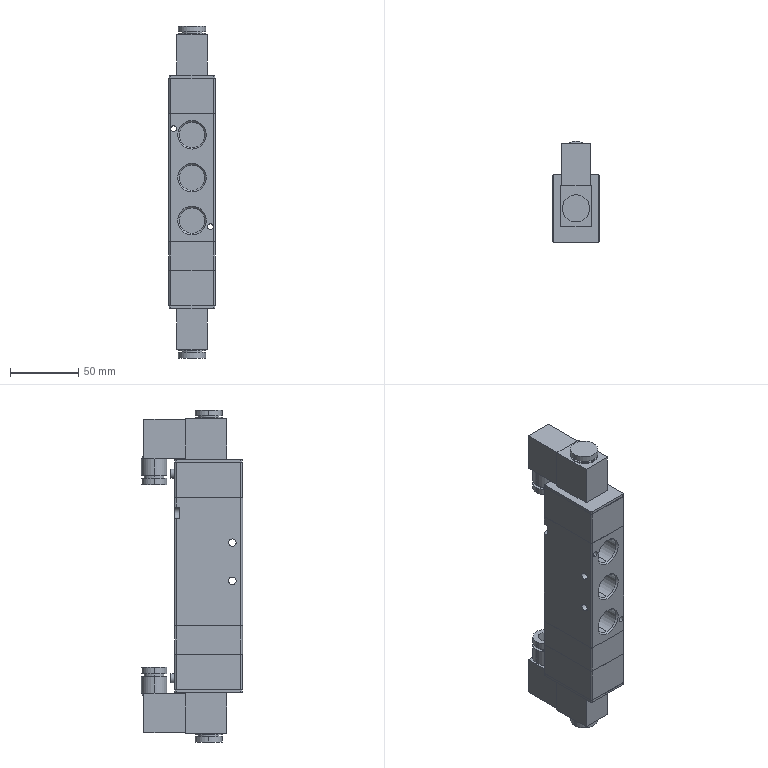Part | SolidWorks | features BaseBody 1 | 1 solid | 168 faces | box 34 x 74.3 x 243.8 mm | volume 351634 mm3 | cylinder 78 | plane 78 | cone 12 | commonest cylinder face diameters 2.4 x26 18.631 x10 15 x8 18.6 x8 20 x8 4.3 x4